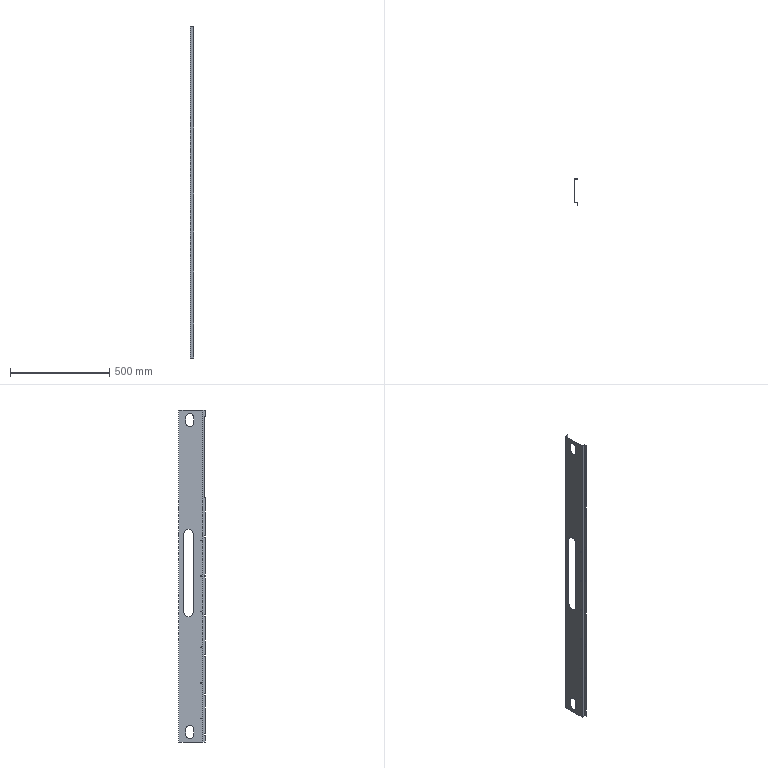Part | STEP file | RJWD-DY-0102_X2_5DE667DC95E8_49 | 1 solid | 82 faces | box 18.5 x 134.2 x 1677 mm | volume 204085 mm3 | plane 58 | cylinder 24 | commonest cylinder face diameters 3.3 x12 40 x4 0.4 x3 2 x3 50 x2